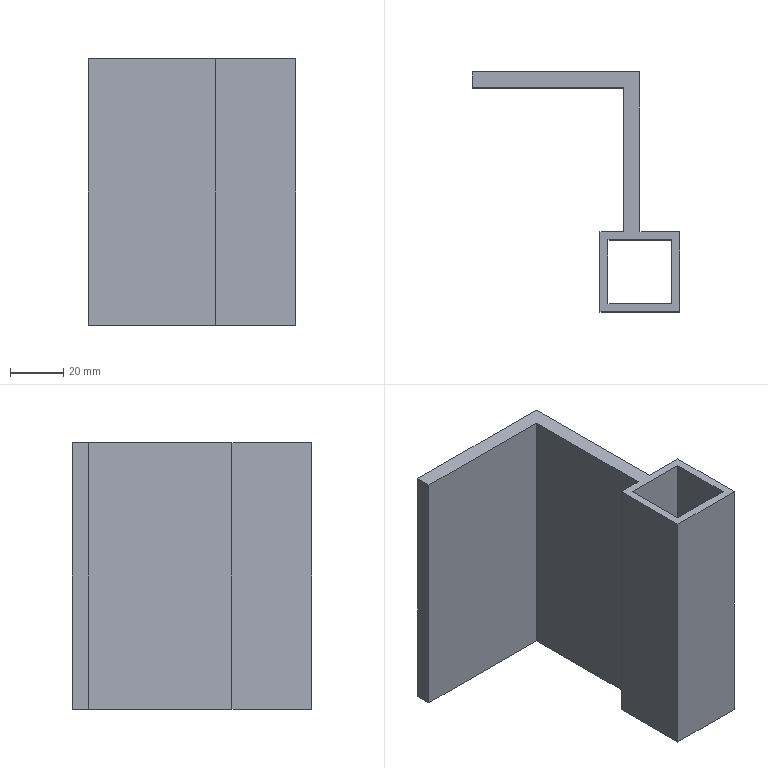Part | NX | features solid 2 | 1 solid | 16 faces | box 78 x 90 x 100 mm | volume 102600 mm3 | plane 16
STEP:
#1=CARTESIAN_POINT('',(-292.,-910.,-205.));
#2=VERTEX_POINT('',#1);
#3=CARTESIAN_POINT('',(-307.,-910.,-205.));
#4=VERTEX_POINT('',#3);
#5=CARTESIAN_POINT('',(-292.,-910.,-205.));
#6=DIRECTION('',(-1.,0.,0.));
#7=VECTOR('',#6,1000.);
#8=LINE('',#5,#7);
#9=EDGE_CURVE('',#2,#4,#8,.T.);
#10=ORIENTED_EDGE('',*,*,#9,.T.);
#11=CARTESIAN_POINT('',(-307.,-910.,-105.));
#12=VERTEX_POINT('',#11);
#13=CARTESIAN_POINT('',(-307.,-910.,-205.));
#14=DIRECTION('',(0.,0.,1.));
#15=VECTOR('',#14,1000.);
#16=LINE('',#13,#15);
#17=EDGE_CURVE('',#4,#12,#16,.T.);
#18=ORIENTED_EDGE('',*,*,#17,.T.);
#19=CARTESIAN_POINT('',(-292.,-910.,-105.));
#20=VERTEX_POINT('',#19);
#21=CARTESIAN_POINT('',(-292.,-910.,-105.));
#22=DIRECTION('',(-1.,0.,0.));
#23=VECTOR('',#22,1000.);
#24=LINE('',#21,#23);
#25=EDGE_CURVE('',#20,#12,#24,.T.);
#26=ORIENTED_EDGE('',*,*,#25,.F.);
#27=CARTESIAN_POINT('',(-292.,-910.,-205.));
#28=DIRECTION('',(0.,0.,1.));
#29=VECTOR('',#28,1000.);
#30=LINE('',#27,#29);
#31=EDGE_CURVE('',#2,#20,#30,.T.);
#32=ORIENTED_EDGE('',*,*,#31,.F.);
#33=EDGE_LOOP('',(#10,#18,#26,#32));
#34=FACE_BOUND('',#33,.T.);
#35=CARTESIAN_POINT('',(-292.,-910.,-205.));
#36=DIRECTION('',(0.,1.,0.));
#37=DIRECTION('',(0.,0.,-1.));
#38=AXIS2_PLACEMENT_3D('',#35,#36,#37);
#39=PLANE('',#38);
#40=ADVANCED_FACE('',(#34),#39,.T.);
#41=CARTESIAN_POINT('',(-319.,-913.,-105.));
#42=VERTEX_POINT('',#41);
#43=CARTESIAN_POINT('',(-319.,-937.,-105.));
#44=VERTEX_POINT('',#43);
#45=CARTESIAN_POINT('',(-319.,-910.,-105.));
#46=DIRECTION('',(0.,-1.,0.));
#47=VECTOR('',#46,1000.);
#48=LINE('',#45,#47);
#49=EDGE_CURVE('',#42,#44,#48,.T.);
#50=ORIENTED_EDGE('',*,*,#49,.F.);
#51=CARTESIAN_POINT('',(-295.,-913.,-105.));
#52=VERTEX_POINT('',#51);
#53=CARTESIAN_POINT('',(-292.,-913.,-105.));
#54=DIRECTION('',(-1.,0.,0.));
#55=VECTOR('',#54,1000.);
#56=LINE('',#53,#55);
#57=EDGE_CURVE('',#52,#42,#56,.T.);
#58=ORIENTED_EDGE('',*,*,#57,.F.);
#59=CARTESIAN_POINT('',(-295.,-937.,-105.));
#60=VERTEX_POINT('',#59);
#61=CARTESIAN_POINT('',(-295.,-940.,-105.));
#62=DIRECTION('',(0.,1.,0.));
#63=VECTOR('',#62,1000.);
#64=LINE('',#61,#63);
#65=EDGE_CURVE('',#60,#52,#64,.T.);
#66=ORIENTED_EDGE('',*,*,#65,.F.);
#67=CARTESIAN_POINT('',(-322.,-937.,-105.));
#68=DIRECTION('',(1.,0.,0.));
#69=VECTOR('',#68,1000.);
#70=LINE('',#67,#69);
#71=EDGE_CURVE('',#44,#60,#70,.T.);
#72=ORIENTED_EDGE('',*,*,#71,.F.);
#73=EDGE_LOOP('',(#50,#58,#66,#72));
#74=FACE_BOUND('',#73,.T.);
#75=CARTESIAN_POINT('',(-322.,-910.,-105.));
#76=VERTEX_POINT('',#75);
#77=CARTESIAN_POINT('',(-322.,-940.,-105.));
#78=VERTEX_POINT('',#77);
#79=CARTESIAN_POINT('',(-322.,-910.,-105.));
#80=DIRECTION('',(0.,-1.,0.));
#81=VECTOR('',#80,1000.);
#82=LINE('',#79,#81);
#83=EDGE_CURVE('',#76,#78,#82,.T.);
#84=ORIENTED_EDGE('',*,*,#83,.T.);
#85=CARTESIAN_POINT('',(-292.,-940.,-105.));
#86=VERTEX_POINT('',#85);
#87=CARTESIAN_POINT('',(-322.,-940.,-105.));
#88=DIRECTION('',(1.,0.,0.));
#89=VECTOR('',#88,1000.);
#90=LINE('',#87,#89);
#91=EDGE_CURVE('',#78,#86,#90,.T.);
#92=ORIENTED_EDGE('',*,*,#91,.T.);
#93=CARTESIAN_POINT('',(-292.,-940.,-105.));
#94=DIRECTION('',(0.,1.,0.));
#95=VECTOR('',#94,1000.);
#96=LINE('',#93,#95);
#97=EDGE_CURVE('',#86,#20,#96,.T.);
#98=ORIENTED_EDGE('',*,*,#97,.T.);
#99=ORIENTED_EDGE('',*,*,#25,.T.);
#100=CARTESIAN_POINT('',(-307.,-850.,-105.));
#101=VERTEX_POINT('',#100);
#102=CARTESIAN_POINT('',(-307.,-910.,-105.));
#103=DIRECTION('',(0.,1.,0.));
#104=VECTOR('',#103,1000.);
#105=LINE('',#102,#104);
#106=EDGE_CURVE('',#12,#101,#105,.T.);
#107=ORIENTED_EDGE('',*,*,#106,.T.);
#108=CARTESIAN_POINT('',(-370.,-850.,-105.));
#109=VERTEX_POINT('',#108);
#110=CARTESIAN_POINT('',(-322.,-850.,-105.));
#111=DIRECTION('',(1.,0.,0.));
#112=VECTOR('',#111,1000.);
#113=LINE('',#110,#112);
#114=EDGE_CURVE('',#101,#109,#113,.F.);
#115=ORIENTED_EDGE('',*,*,#114,.T.);
#116=CARTESIAN_POINT('',(-370.,-856.,-105.));
#117=VERTEX_POINT('',#116);
#118=CARTESIAN_POINT('',(-370.,-847.,-105.));
#119=DIRECTION('',(0.,1.,0.));
#120=VECTOR('',#119,1000.);
#121=LINE('',#118,#120);
#122=EDGE_CURVE('',#109,#117,#121,.F.);
#123=ORIENTED_EDGE('',*,*,#122,.T.);
#124=CARTESIAN_POINT('',(-313.,-856.,-105.));
#125=VERTEX_POINT('',#124);
#126=CARTESIAN_POINT('',(-322.,-856.,-105.));
#127=DIRECTION('',(1.,0.,0.));
#128=VECTOR('',#127,1000.);
#129=LINE('',#126,#128);
#130=EDGE_CURVE('',#125,#117,#129,.F.);
#131=ORIENTED_EDGE('',*,*,#130,.F.);
#132=CARTESIAN_POINT('',(-313.,-910.,-105.));
#133=VERTEX_POINT('',#132);
#134=CARTESIAN_POINT('',(-313.,-910.,-105.));
#135=DIRECTION('',(0.,1.,0.));
#136=VECTOR('',#135,1000.);
#137=LINE('',#134,#136);
#138=EDGE_CURVE('',#133,#125,#137,.T.);
#139=ORIENTED_EDGE('',*,*,#138,.F.);
#140=CARTESIAN_POINT('',(-292.,-910.,-105.));
#141=DIRECTION('',(-1.,0.,0.));
#142=VECTOR('',#141,1000.);
#143=LINE('',#140,#142);
#144=EDGE_CURVE('',#133,#76,#143,.T.);
#145=ORIENTED_EDGE('',*,*,#144,.T.);
#146=EDGE_LOOP('',(#84,#92,#98,#99,#107,#115,#123,#131,#139,#145));
#147=FACE_BOUND('',#146,.T.);
#148=CARTESIAN_POINT('',(-322.,-910.,-105.));
#149=DIRECTION('',(0.,0.,-1.));
#150=DIRECTION('',(0.,-1.,0.));
#151=AXIS2_PLACEMENT_3D('',#148,#149,#150);
#152=PLANE('',#151);
#153=ADVANCED_FACE('',(#74,#147),#152,.F.);
#154=CARTESIAN_POINT('',(-295.,-937.,-205.));
#155=VERTEX_POINT('',#154);
#156=CARTESIAN_POINT('',(-295.,-913.,-205.));
#157=VERTEX_POINT('',#156);
#158=CARTESIAN_POINT('',(-295.,-940.,-205.));
#159=DIRECTION('',(0.,1.,0.));
#160=VECTOR('',#159,1000.);
#161=LINE('',#158,#160);
#162=EDGE_CURVE('',#155,#157,#161,.T.);
#163=ORIENTED_EDGE('',*,*,#162,.T.);
#164=CARTESIAN_POINT('',(-319.,-913.,-205.));
#165=VERTEX_POINT('',#164);
#166=CARTESIAN_POINT('',(-292.,-913.,-205.));
#167=DIRECTION('',(-1.,0.,0.));
#168=VECTOR('',#167,1000.);
#169=LINE('',#166,#168);
#170=EDGE_CURVE('',#157,#165,#169,.T.);
#171=ORIENTED_EDGE('',*,*,#170,.T.);
#172=CARTESIAN_POINT('',(-319.,-937.,-205.));
#173=VERTEX_POINT('',#172);
#174=CARTESIAN_POINT('',(-319.,-910.,-205.));
#175=DIRECTION('',(0.,-1.,0.));
#176=VECTOR('',#175,1000.);
#177=LINE('',#174,#176);
#178=EDGE_CURVE('',#165,#173,#177,.T.);
#179=ORIENTED_EDGE('',*,*,#178,.T.);
#180=CARTESIAN_POINT('',(-322.,-937.,-205.));
#181=DIRECTION('',(1.,0.,0.));
#182=VECTOR('',#181,1000.);
#183=LINE('',#180,#182);
#184=EDGE_CURVE('',#173,#155,#183,.T.);
#185=ORIENTED_EDGE('',*,*,#184,.T.);
#186=EDGE_LOOP('',(#163,#171,#179,#185));
#187=FACE_BOUND('',#186,.T.);
#188=CARTESIAN_POINT('',(-292.,-940.,-205.));
#189=VERTEX_POINT('',#188);
#190=CARTESIAN_POINT('',(-292.,-940.,-205.));
#191=DIRECTION('',(0.,1.,0.));
#192=VECTOR('',#191,1000.);
#193=LINE('',#190,#192);
#194=EDGE_CURVE('',#189,#2,#193,.T.);
#195=ORIENTED_EDGE('',*,*,#194,.F.);
#196=CARTESIAN_POINT('',(-322.,-940.,-205.));
#197=VERTEX_POINT('',#196);
#198=CARTESIAN_POINT('',(-322.,-940.,-205.));
#199=DIRECTION('',(1.,0.,0.));
#200=VECTOR('',#199,1000.);
#201=LINE('',#198,#200);
#202=EDGE_CURVE('',#197,#189,#201,.T.);
#203=ORIENTED_EDGE('',*,*,#202,.F.);
#204=CARTESIAN_POINT('',(-322.,-910.,-205.));
#205=VERTEX_POINT('',#204);
#206=CARTESIAN_POINT('',(-322.,-910.,-205.));
#207=DIRECTION('',(0.,-1.,0.));
#208=VECTOR('',#207,1000.);
#209=LINE('',#206,#208);
#210=EDGE_CURVE('',#205,#197,#209,.T.);
#211=ORIENTED_EDGE('',*,*,#210,.F.);
#212=CARTESIAN_POINT('',(-313.,-910.,-205.));
#213=VERTEX_POINT('',#212);
#214=CARTESIAN_POINT('',(-292.,-910.,-205.));
#215=DIRECTION('',(-1.,0.,0.));
#216=VECTOR('',#215,1000.);
#217=LINE('',#214,#216);
#218=EDGE_CURVE('',#213,#205,#217,.T.);
#219=ORIENTED_EDGE('',*,*,#218,.F.);
#220=CARTESIAN_POINT('',(-313.,-856.,-205.));
#221=VERTEX_POINT('',#220);
#222=CARTESIAN_POINT('',(-313.,-910.,-205.));
#223=DIRECTION('',(0.,1.,0.));
#224=VECTOR('',#223,1000.);
#225=LINE('',#222,#224);
#226=EDGE_CURVE('',#213,#221,#225,.T.);
#227=ORIENTED_EDGE('',*,*,#226,.T.);
#228=CARTESIAN_POINT('',(-370.,-856.,-205.));
#229=VERTEX_POINT('',#228);
#230=CARTESIAN_POINT('',(-307.,-856.,-205.));
#231=DIRECTION('',(-1.,0.,0.));
#232=VECTOR('',#231,1000.);
#233=LINE('',#230,#232);
#234=EDGE_CURVE('',#221,#229,#233,.T.);
#235=ORIENTED_EDGE('',*,*,#234,.T.);
#236=CARTESIAN_POINT('',(-370.,-850.,-205.));
#237=VERTEX_POINT('',#236);
#238=CARTESIAN_POINT('',(-370.,-847.,-205.));
#239=DIRECTION('',(0.,1.,0.));
#240=VECTOR('',#239,1000.);
#241=LINE('',#238,#240);
#242=EDGE_CURVE('',#237,#229,#241,.F.);
#243=ORIENTED_EDGE('',*,*,#242,.F.);
#244=CARTESIAN_POINT('',(-307.,-850.,-205.));
#245=VERTEX_POINT('',#244);
#246=CARTESIAN_POINT('',(-307.,-850.,-205.));
#247=DIRECTION('',(-1.,0.,0.));
#248=VECTOR('',#247,1000.);
#249=LINE('',#246,#248);
#250=EDGE_CURVE('',#245,#237,#249,.T.);
#251=ORIENTED_EDGE('',*,*,#250,.F.);
#252=CARTESIAN_POINT('',(-307.,-910.,-205.));
#253=DIRECTION('',(0.,1.,0.));
#254=VECTOR('',#253,1000.);
#255=LINE('',#252,#254);
#256=EDGE_CURVE('',#4,#245,#255,.T.);
#257=ORIENTED_EDGE('',*,*,#256,.F.);
#258=ORIENTED_EDGE('',*,*,#9,.F.);
#259=EDGE_LOOP('',(#195,#203,#211,#219,#227,#235,#243,#251,#257,#258));
#260=FACE_BOUND('',#259,.T.);
#261=CARTESIAN_POINT('',(-292.,-940.,-205.));
#262=DIRECTION('',(0.,0.,-1.));
#263=DIRECTION('',(0.,1.,0.));
#264=AXIS2_PLACEMENT_3D('',#261,#262,#263);
#265=PLANE('',#264);
#266=ADVANCED_FACE('',(#187,#260),#265,.T.);
#267=ORIENTED_EDGE('',*,*,#57,.T.);
#268=CARTESIAN_POINT('',(-319.,-913.,-205.));
#269=DIRECTION('',(0.,0.,1.));
#270=VECTOR('',#269,1000.);
#271=LINE('',#268,#270);
#272=EDGE_CURVE('',#165,#42,#271,.T.);
#273=ORIENTED_EDGE('',*,*,#272,.F.);
#274=ORIENTED_EDGE('',*,*,#170,.F.);
#275=CARTESIAN_POINT('',(-295.,-913.,-205.));
#276=DIRECTION('',(0.,0.,1.));
#277=VECTOR('',#276,1000.);
#278=LINE('',#275,#277);
#279=EDGE_CURVE('',#157,#52,#278,.T.);
#280=ORIENTED_EDGE('',*,*,#279,.T.);
#281=EDGE_LOOP('',(#267,#273,#274,#280));
#282=FACE_BOUND('',#281,.T.);
#283=CARTESIAN_POINT('',(-292.,-913.,-205.));
#284=DIRECTION('',(0.,1.,0.));
#285=DIRECTION('',(0.,0.,-1.));
#286=AXIS2_PLACEMENT_3D('',#283,#284,#285);
#287=PLANE('',#286);
#288=ADVANCED_FACE('',(#282),#287,.F.);
#289=ORIENTED_EDGE('',*,*,#65,.T.);
#290=ORIENTED_EDGE('',*,*,#279,.F.);
#291=ORIENTED_EDGE('',*,*,#162,.F.);
#292=CARTESIAN_POINT('',(-295.,-937.,-205.));
#293=DIRECTION('',(0.,0.,1.));
#294=VECTOR('',#293,1000.);
#295=LINE('',#292,#294);
#296=EDGE_CURVE('',#155,#60,#295,.T.);
#297=ORIENTED_EDGE('',*,*,#296,.T.);
#298=EDGE_LOOP('',(#289,#290,#291,#297));
#299=FACE_BOUND('',#298,.T.);
#300=CARTESIAN_POINT('',(-295.,-940.,-205.));
#301=DIRECTION('',(1.,0.,0.));
#302=DIRECTION('',(0.,1.,0.));
#303=AXIS2_PLACEMENT_3D('',#300,#301,#302);
#304=PLANE('',#303);
#305=ADVANCED_FACE('',(#299),#304,.F.);
#306=ORIENTED_EDGE('',*,*,#71,.T.);
#307=ORIENTED_EDGE('',*,*,#296,.F.);
#308=ORIENTED_EDGE('',*,*,#184,.F.);
#309=CARTESIAN_POINT('',(-319.,-937.,-205.));
#310=DIRECTION('',(0.,0.,1.));
#311=VECTOR('',#310,1000.);
#312=LINE('',#309,#311);
#313=EDGE_CURVE('',#173,#44,#312,.T.);
#314=ORIENTED_EDGE('',*,*,#313,.T.);
#315=EDGE_LOOP('',(#306,#307,#308,#314));
#316=FACE_BOUND('',#315,.T.);
#317=CARTESIAN_POINT('',(-322.,-937.,-205.));
#318=DIRECTION('',(0.,-1.,0.));
#319=DIRECTION('',(1.,0.,0.));
#320=AXIS2_PLACEMENT_3D('',#317,#318,#319);
#321=PLANE('',#320);
#322=ADVANCED_FACE('',(#316),#321,.F.);
#323=ORIENTED_EDGE('',*,*,#49,.T.);
#324=ORIENTED_EDGE('',*,*,#313,.F.);
#325=ORIENTED_EDGE('',*,*,#178,.F.);
#326=ORIENTED_EDGE('',*,*,#272,.T.);
#327=EDGE_LOOP('',(#323,#324,#325,#326));
#328=FACE_BOUND('',#327,.T.);
#329=CARTESIAN_POINT('',(-319.,-910.,-205.));
#330=DIRECTION('',(-1.,0.,0.));
#331=DIRECTION('',(0.,0.,-1.));
#332=AXIS2_PLACEMENT_3D('',#329,#330,#331);
#333=PLANE('',#332);
#334=ADVANCED_FACE('',(#328),#333,.F.);
#335=CARTESIAN_POINT('',(-313.,-910.,-205.));
#336=DIRECTION('',(0.,0.,1.));
#337=VECTOR('',#336,1000.);
#338=LINE('',#335,#337);
#339=EDGE_CURVE('',#213,#133,#338,.T.);
#340=ORIENTED_EDGE('',*,*,#339,.F.);
#341=ORIENTED_EDGE('',*,*,#218,.T.);
#342=CARTESIAN_POINT('',(-322.,-910.,-205.));
#343=DIRECTION('',(0.,0.,1.));
#344=VECTOR('',#343,1000.);
#345=LINE('',#342,#344);
#346=EDGE_CURVE('',#205,#76,#345,.T.);
#347=ORIENTED_EDGE('',*,*,#346,.T.);
#348=ORIENTED_EDGE('',*,*,#144,.F.);
#349=EDGE_LOOP('',(#340,#341,#347,#348));
#350=FACE_BOUND('',#349,.T.);
#351=CARTESIAN_POINT('',(-292.,-910.,-205.));
#352=DIRECTION('',(0.,1.,0.));
#353=DIRECTION('',(0.,0.,-1.));
#354=AXIS2_PLACEMENT_3D('',#351,#352,#353);
#355=PLANE('',#354);
#356=ADVANCED_FACE('',(#350),#355,.T.);
#357=ORIENTED_EDGE('',*,*,#97,.F.);
#358=CARTESIAN_POINT('',(-292.,-940.,-205.));
#359=DIRECTION('',(0.,0.,1.));
#360=VECTOR('',#359,1000.);
#361=LINE('',#358,#360);
#362=EDGE_CURVE('',#189,#86,#361,.T.);
#363=ORIENTED_EDGE('',*,*,#362,.F.);
#364=ORIENTED_EDGE('',*,*,#194,.T.);
#365=ORIENTED_EDGE('',*,*,#31,.T.);
#366=EDGE_LOOP('',(#357,#363,#364,#365));
#367=FACE_BOUND('',#366,.T.);
#368=CARTESIAN_POINT('',(-292.,-940.,-205.));
#369=DIRECTION('',(1.,0.,0.));
#370=DIRECTION('',(0.,1.,0.));
#371=AXIS2_PLACEMENT_3D('',#368,#369,#370);
#372=PLANE('',#371);
#373=ADVANCED_FACE('',(#367),#372,.T.);
#374=ORIENTED_EDGE('',*,*,#91,.F.);
#375=CARTESIAN_POINT('',(-322.,-940.,-205.));
#376=DIRECTION('',(0.,0.,1.));
#377=VECTOR('',#376,1000.);
#378=LINE('',#375,#377);
#379=EDGE_CURVE('',#197,#78,#378,.T.);
#380=ORIENTED_EDGE('',*,*,#379,.F.);
#381=ORIENTED_EDGE('',*,*,#202,.T.);
#382=ORIENTED_EDGE('',*,*,#362,.T.);
#383=EDGE_LOOP('',(#374,#380,#381,#382));
#384=FACE_BOUND('',#383,.T.);
#385=CARTESIAN_POINT('',(-322.,-940.,-205.));
#386=DIRECTION('',(0.,-1.,0.));
#387=DIRECTION('',(1.,0.,0.));
#388=AXIS2_PLACEMENT_3D('',#385,#386,#387);
#389=PLANE('',#388);
#390=ADVANCED_FACE('',(#384),#389,.T.);
#391=ORIENTED_EDGE('',*,*,#83,.F.);
#392=ORIENTED_EDGE('',*,*,#346,.F.);
#393=ORIENTED_EDGE('',*,*,#210,.T.);
#394=ORIENTED_EDGE('',*,*,#379,.T.);
#395=EDGE_LOOP('',(#391,#392,#393,#394));
#396=FACE_BOUND('',#395,.T.);
#397=CARTESIAN_POINT('',(-322.,-910.,-205.));
#398=DIRECTION('',(-1.,0.,0.));
#399=DIRECTION('',(0.,0.,-1.));
#400=AXIS2_PLACEMENT_3D('',#397,#398,#399);
#401=PLANE('',#400);
#402=ADVANCED_FACE('',(#396),#401,.T.);
#403=ORIENTED_EDGE('',*,*,#242,.T.);
#404=CARTESIAN_POINT('',(-370.,-856.,-205.));
#405=DIRECTION('',(0.,0.,-1.));
#406=VECTOR('',#405,1000.);
#407=LINE('',#404,#406);
#408=EDGE_CURVE('',#229,#117,#407,.F.);
#409=ORIENTED_EDGE('',*,*,#408,.T.);
#410=ORIENTED_EDGE('',*,*,#122,.F.);
#411=CARTESIAN_POINT('',(-370.,-850.,-205.));
#412=DIRECTION('',(0.,0.,-1.));
#413=VECTOR('',#412,1000.);
#414=LINE('',#411,#413);
#415=EDGE_CURVE('',#237,#109,#414,.F.);
#416=ORIENTED_EDGE('',*,*,#415,.F.);
#417=EDGE_LOOP('',(#403,#409,#410,#416));
#418=FACE_BOUND('',#417,.T.);
#419=CARTESIAN_POINT('',(-370.,-847.,-205.));
#420=DIRECTION('',(-1.,0.,0.));
#421=DIRECTION('',(0.,0.,1.));
#422=AXIS2_PLACEMENT_3D('',#419,#420,#421);
#423=PLANE('',#422);
#424=ADVANCED_FACE('',(#418),#423,.T.);
#425=ORIENTED_EDGE('',*,*,#138,.T.);
#426=CARTESIAN_POINT('',(-313.,-856.,-205.));
#427=DIRECTION('',(0.,0.,1.));
#428=VECTOR('',#427,1000.);
#429=LINE('',#426,#428);
#430=EDGE_CURVE('',#221,#125,#429,.T.);
#431=ORIENTED_EDGE('',*,*,#430,.F.);
#432=ORIENTED_EDGE('',*,*,#226,.F.);
#433=ORIENTED_EDGE('',*,*,#339,.T.);
#434=EDGE_LOOP('',(#425,#431,#432,#433));
#435=FACE_BOUND('',#434,.T.);
#436=CARTESIAN_POINT('',(-313.,-910.,-205.));
#437=DIRECTION('',(1.,0.,0.));
#438=DIRECTION('',(0.,1.,0.));
#439=AXIS2_PLACEMENT_3D('',#436,#437,#438);
#440=PLANE('',#439);
#441=ADVANCED_FACE('',(#435),#440,.F.);
#442=ORIENTED_EDGE('',*,*,#130,.T.);
#443=ORIENTED_EDGE('',*,*,#408,.F.);
#444=ORIENTED_EDGE('',*,*,#234,.F.);
#445=ORIENTED_EDGE('',*,*,#430,.T.);
#446=EDGE_LOOP('',(#442,#443,#444,#445));
#447=FACE_BOUND('',#446,.T.);
#448=CARTESIAN_POINT('',(-307.,-856.,-205.));
#449=DIRECTION('',(0.,1.,0.));
#450=DIRECTION('',(0.,0.,-1.));
#451=AXIS2_PLACEMENT_3D('',#448,#449,#450);
#452=PLANE('',#451);
#453=ADVANCED_FACE('',(#447),#452,.F.);
#454=ORIENTED_EDGE('',*,*,#106,.F.);
#455=ORIENTED_EDGE('',*,*,#17,.F.);
#456=ORIENTED_EDGE('',*,*,#256,.T.);
#457=CARTESIAN_POINT('',(-307.,-850.,-205.));
#458=DIRECTION('',(0.,0.,1.));
#459=VECTOR('',#458,1000.);
#460=LINE('',#457,#459);
#461=EDGE_CURVE('',#245,#101,#460,.T.);
#462=ORIENTED_EDGE('',*,*,#461,.T.);
#463=EDGE_LOOP('',(#454,#455,#456,#462));
#464=FACE_BOUND('',#463,.T.);
#465=CARTESIAN_POINT('',(-307.,-910.,-205.));
#466=DIRECTION('',(1.,0.,0.));
#467=DIRECTION('',(0.,1.,0.));
#468=AXIS2_PLACEMENT_3D('',#465,#466,#467);
#469=PLANE('',#468);
#470=ADVANCED_FACE('',(#464),#469,.T.);
#471=ORIENTED_EDGE('',*,*,#114,.F.);
#472=ORIENTED_EDGE('',*,*,#461,.F.);
#473=ORIENTED_EDGE('',*,*,#250,.T.);
#474=ORIENTED_EDGE('',*,*,#415,.T.);
#475=EDGE_LOOP('',(#471,#472,#473,#474));
#476=FACE_BOUND('',#475,.T.);
#477=CARTESIAN_POINT('',(-307.,-850.,-205.));
#478=DIRECTION('',(0.,1.,0.));
#479=DIRECTION('',(0.,0.,-1.));
#480=AXIS2_PLACEMENT_3D('',#477,#478,#479);
#481=PLANE('',#480);
#482=ADVANCED_FACE('',(#476),#481,.T.);
#483=CLOSED_SHELL('',(#40,#153,#266,#288,#305,#322,#334,#356,#373,#390,#402,#424,#441,#453,#470,#482));
#484=MANIFOLD_SOLID_BREP('',#483);
#485=(LENGTH_UNIT()NAMED_UNIT(*)SI_UNIT(.MILLI.,.METRE.));
#486=UNCERTAINTY_MEASURE_WITH_UNIT(LENGTH_MEASURE(0.00001),#485,'','');
#487=(NAMED_UNIT(*)PLANE_ANGLE_UNIT()SI_UNIT($,.RADIAN.));
#488=(NAMED_UNIT(*)SI_UNIT($,.STERADIAN.)SOLID_ANGLE_UNIT());
#489=(GEOMETRIC_REPRESENTATION_CONTEXT(3)GLOBAL_UNCERTAINTY_ASSIGNED_CONTEXT((#486))GLOBAL_UNIT_ASSIGNED_CONTEXT((#485,#487,#488))REPRESENTATION_CONTEXT('',''));
#490=ADVANCED_BREP_SHAPE_REPRESENTATION('',(#484),#489);